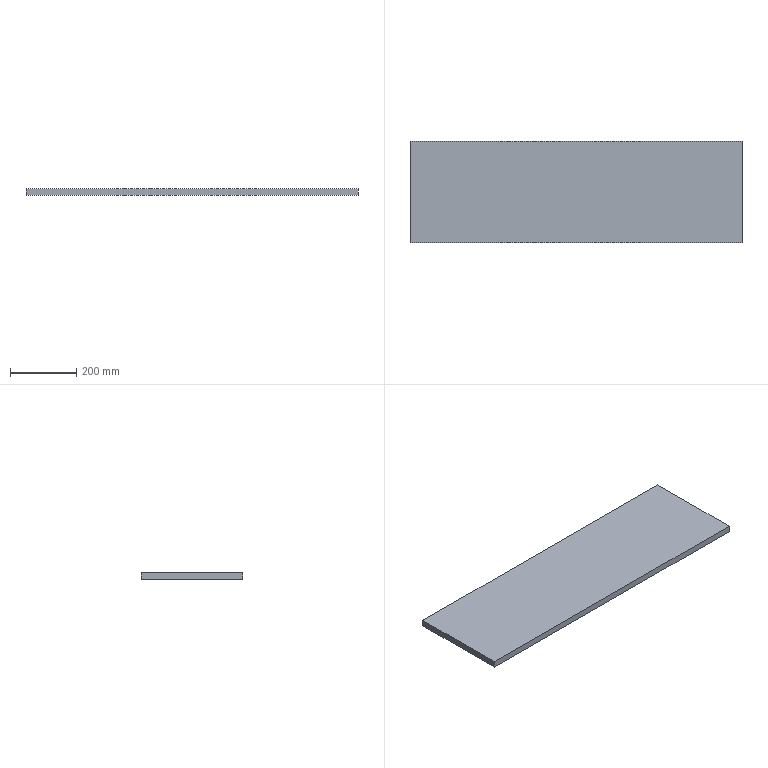Part | SolidWorks | features BaseBody 1 | 1 solid | 6 faces | box 1000 x 305 x 20 mm | volume 6100000 mm3 | plane 6
STEP:
#1=CARTESIAN_POINT('',(2389.703,1856.615,0.));
#2=VERTEX_POINT('',#1);
#3=CARTESIAN_POINT('',(2389.703,1551.615,0.));
#4=VERTEX_POINT('',#3);
#5=CARTESIAN_POINT('',(2389.703,1551.615,0.));
#6=DIRECTION('',(0.,-1.,0.));
#7=VECTOR('',#6,1000.);
#8=LINE('',#5,#7);
#9=EDGE_CURVE('',#2,#4,#8,.T.);
#10=ORIENTED_EDGE('',*,*,#9,.T.);
#11=CARTESIAN_POINT('',(2389.703,1551.615,20.));
#12=VERTEX_POINT('',#11);
#13=CARTESIAN_POINT('',(2389.703,1551.615,20.));
#14=DIRECTION('',(0.,0.,-1.));
#15=VECTOR('',#14,1000.);
#16=LINE('',#13,#15);
#17=EDGE_CURVE('',#12,#4,#16,.T.);
#18=ORIENTED_EDGE('',*,*,#17,.F.);
#19=CARTESIAN_POINT('',(2389.703,1856.615,20.));
#20=VERTEX_POINT('',#19);
#21=CARTESIAN_POINT('',(2389.703,1551.615,20.));
#22=DIRECTION('',(0.,-1.,0.));
#23=VECTOR('',#22,1000.);
#24=LINE('',#21,#23);
#25=EDGE_CURVE('',#20,#12,#24,.T.);
#26=ORIENTED_EDGE('',*,*,#25,.F.);
#27=CARTESIAN_POINT('',(2389.703,1856.615,20.));
#28=DIRECTION('',(0.,0.,-1.));
#29=VECTOR('',#28,1000.);
#30=LINE('',#27,#29);
#31=EDGE_CURVE('',#20,#2,#30,.T.);
#32=ORIENTED_EDGE('',*,*,#31,.T.);
#33=EDGE_LOOP('',(#10,#18,#26,#32));
#34=FACE_OUTER_BOUND('',#33,.T.);
#35=CARTESIAN_POINT('',(2389.703,1551.615,20.));
#36=DIRECTION('',(1.,0.,0.));
#37=DIRECTION('',(0.,0.,-1.));
#38=AXIS2_PLACEMENT_3D('',#35,#36,#37);
#39=PLANE('',#38);
#40=ADVANCED_FACE('',(#34),#39,.F.);
#41=CARTESIAN_POINT('',(3389.703,1551.615,0.));
#42=VERTEX_POINT('',#41);
#43=CARTESIAN_POINT('',(3389.703,1551.615,0.));
#44=DIRECTION('',(1.,0.,0.));
#45=VECTOR('',#44,1000.);
#46=LINE('',#43,#45);
#47=EDGE_CURVE('',#4,#42,#46,.T.);
#48=ORIENTED_EDGE('',*,*,#47,.T.);
#49=CARTESIAN_POINT('',(3389.703,1551.615,20.));
#50=VERTEX_POINT('',#49);
#51=CARTESIAN_POINT('',(3389.703,1551.615,20.));
#52=DIRECTION('',(0.,0.,-1.));
#53=VECTOR('',#52,1000.);
#54=LINE('',#51,#53);
#55=EDGE_CURVE('',#50,#42,#54,.T.);
#56=ORIENTED_EDGE('',*,*,#55,.F.);
#57=CARTESIAN_POINT('',(3389.703,1551.615,20.));
#58=DIRECTION('',(1.,0.,0.));
#59=VECTOR('',#58,1000.);
#60=LINE('',#57,#59);
#61=EDGE_CURVE('',#12,#50,#60,.T.);
#62=ORIENTED_EDGE('',*,*,#61,.F.);
#63=ORIENTED_EDGE('',*,*,#17,.T.);
#64=EDGE_LOOP('',(#48,#56,#62,#63));
#65=FACE_OUTER_BOUND('',#64,.T.);
#66=CARTESIAN_POINT('',(3389.703,1551.615,20.));
#67=DIRECTION('',(0.,1.,0.));
#68=DIRECTION('',(0.,0.,1.));
#69=AXIS2_PLACEMENT_3D('',#66,#67,#68);
#70=PLANE('',#69);
#71=ADVANCED_FACE('',(#65),#70,.F.);
#72=CARTESIAN_POINT('',(3389.703,1856.615,0.));
#73=VERTEX_POINT('',#72);
#74=CARTESIAN_POINT('',(3389.703,1856.615,0.));
#75=DIRECTION('',(0.,1.,0.));
#76=VECTOR('',#75,1000.);
#77=LINE('',#74,#76);
#78=EDGE_CURVE('',#42,#73,#77,.T.);
#79=ORIENTED_EDGE('',*,*,#78,.T.);
#80=CARTESIAN_POINT('',(3389.703,1856.615,20.));
#81=VERTEX_POINT('',#80);
#82=CARTESIAN_POINT('',(3389.703,1856.615,20.));
#83=DIRECTION('',(0.,0.,-1.));
#84=VECTOR('',#83,1000.);
#85=LINE('',#82,#84);
#86=EDGE_CURVE('',#81,#73,#85,.T.);
#87=ORIENTED_EDGE('',*,*,#86,.F.);
#88=CARTESIAN_POINT('',(3389.703,1856.615,20.));
#89=DIRECTION('',(0.,1.,0.));
#90=VECTOR('',#89,1000.);
#91=LINE('',#88,#90);
#92=EDGE_CURVE('',#50,#81,#91,.T.);
#93=ORIENTED_EDGE('',*,*,#92,.F.);
#94=ORIENTED_EDGE('',*,*,#55,.T.);
#95=EDGE_LOOP('',(#79,#87,#93,#94));
#96=FACE_OUTER_BOUND('',#95,.T.);
#97=CARTESIAN_POINT('',(3389.703,1856.615,20.));
#98=DIRECTION('',(-1.,0.,0.));
#99=DIRECTION('',(0.,0.,1.));
#100=AXIS2_PLACEMENT_3D('',#97,#98,#99);
#101=PLANE('',#100);
#102=ADVANCED_FACE('',(#96),#101,.F.);
#103=CARTESIAN_POINT('',(2389.703,1856.615,0.));
#104=DIRECTION('',(-1.,0.,0.));
#105=VECTOR('',#104,1000.);
#106=LINE('',#103,#105);
#107=EDGE_CURVE('',#73,#2,#106,.T.);
#108=ORIENTED_EDGE('',*,*,#107,.T.);
#109=ORIENTED_EDGE('',*,*,#31,.F.);
#110=CARTESIAN_POINT('',(2389.703,1856.615,20.));
#111=DIRECTION('',(-1.,0.,0.));
#112=VECTOR('',#111,1000.);
#113=LINE('',#110,#112);
#114=EDGE_CURVE('',#81,#20,#113,.T.);
#115=ORIENTED_EDGE('',*,*,#114,.F.);
#116=ORIENTED_EDGE('',*,*,#86,.T.);
#117=EDGE_LOOP('',(#108,#109,#115,#116));
#118=FACE_OUTER_BOUND('',#117,.T.);
#119=CARTESIAN_POINT('',(2389.703,1856.615,20.));
#120=DIRECTION('',(0.,-1.,0.));
#121=DIRECTION('',(0.,0.,-1.));
#122=AXIS2_PLACEMENT_3D('',#119,#120,#121);
#123=PLANE('',#122);
#124=ADVANCED_FACE('',(#118),#123,.F.);
#125=ORIENTED_EDGE('',*,*,#25,.T.);
#126=ORIENTED_EDGE('',*,*,#61,.T.);
#127=ORIENTED_EDGE('',*,*,#92,.T.);
#128=ORIENTED_EDGE('',*,*,#114,.T.);
#129=EDGE_LOOP('',(#125,#126,#127,#128));
#130=FACE_OUTER_BOUND('',#129,.T.);
#131=CARTESIAN_POINT('',(0.,0.,20.));
#132=DIRECTION('',(0.,0.,-1.));
#133=DIRECTION('',(-1.,0.,0.));
#134=AXIS2_PLACEMENT_3D('',#131,#132,#133);
#135=PLANE('',#134);
#136=ADVANCED_FACE('',(#130),#135,.F.);
#137=ORIENTED_EDGE('',*,*,#9,.F.);
#138=ORIENTED_EDGE('',*,*,#107,.F.);
#139=ORIENTED_EDGE('',*,*,#78,.F.);
#140=ORIENTED_EDGE('',*,*,#47,.F.);
#141=EDGE_LOOP('',(#137,#138,#139,#140));
#142=FACE_OUTER_BOUND('',#141,.T.);
#143=CARTESIAN_POINT('',(0.,0.,0.));
#144=DIRECTION('',(0.,0.,-1.));
#145=DIRECTION('',(-1.,0.,0.));
#146=AXIS2_PLACEMENT_3D('',#143,#144,#145);
#147=PLANE('',#146);
#148=ADVANCED_FACE('',(#142),#147,.T.);
#149=CLOSED_SHELL('',(#40,#71,#102,#124,#136,#148));
#150=MANIFOLD_SOLID_BREP('',#149);
#151=CARTESIAN_POINT('',(0.,0.,0.));
#152=DIRECTION('',(0.,0.,1.));
#153=DIRECTION('',(1.,0.,0.));
#154=AXIS2_PLACEMENT_3D('',#151,#152,#153);
#155=(LENGTH_UNIT()NAMED_UNIT(*)SI_UNIT(.MILLI.,.METRE.));
#156=UNCERTAINTY_MEASURE_WITH_UNIT(LENGTH_MEASURE(0.00001),#155,'','');
#157=(NAMED_UNIT(*)PLANE_ANGLE_UNIT()SI_UNIT($,.RADIAN.));
#158=(NAMED_UNIT(*)SI_UNIT($,.STERADIAN.)SOLID_ANGLE_UNIT());
#159=(GEOMETRIC_REPRESENTATION_CONTEXT(3)GLOBAL_UNCERTAINTY_ASSIGNED_CONTEXT((#156))GLOBAL_UNIT_ASSIGNED_CONTEXT((#155,#157,#158))REPRESENTATION_CONTEXT('',''));
#160=ADVANCED_BREP_SHAPE_REPRESENTATION('',(#150,#154),#159);